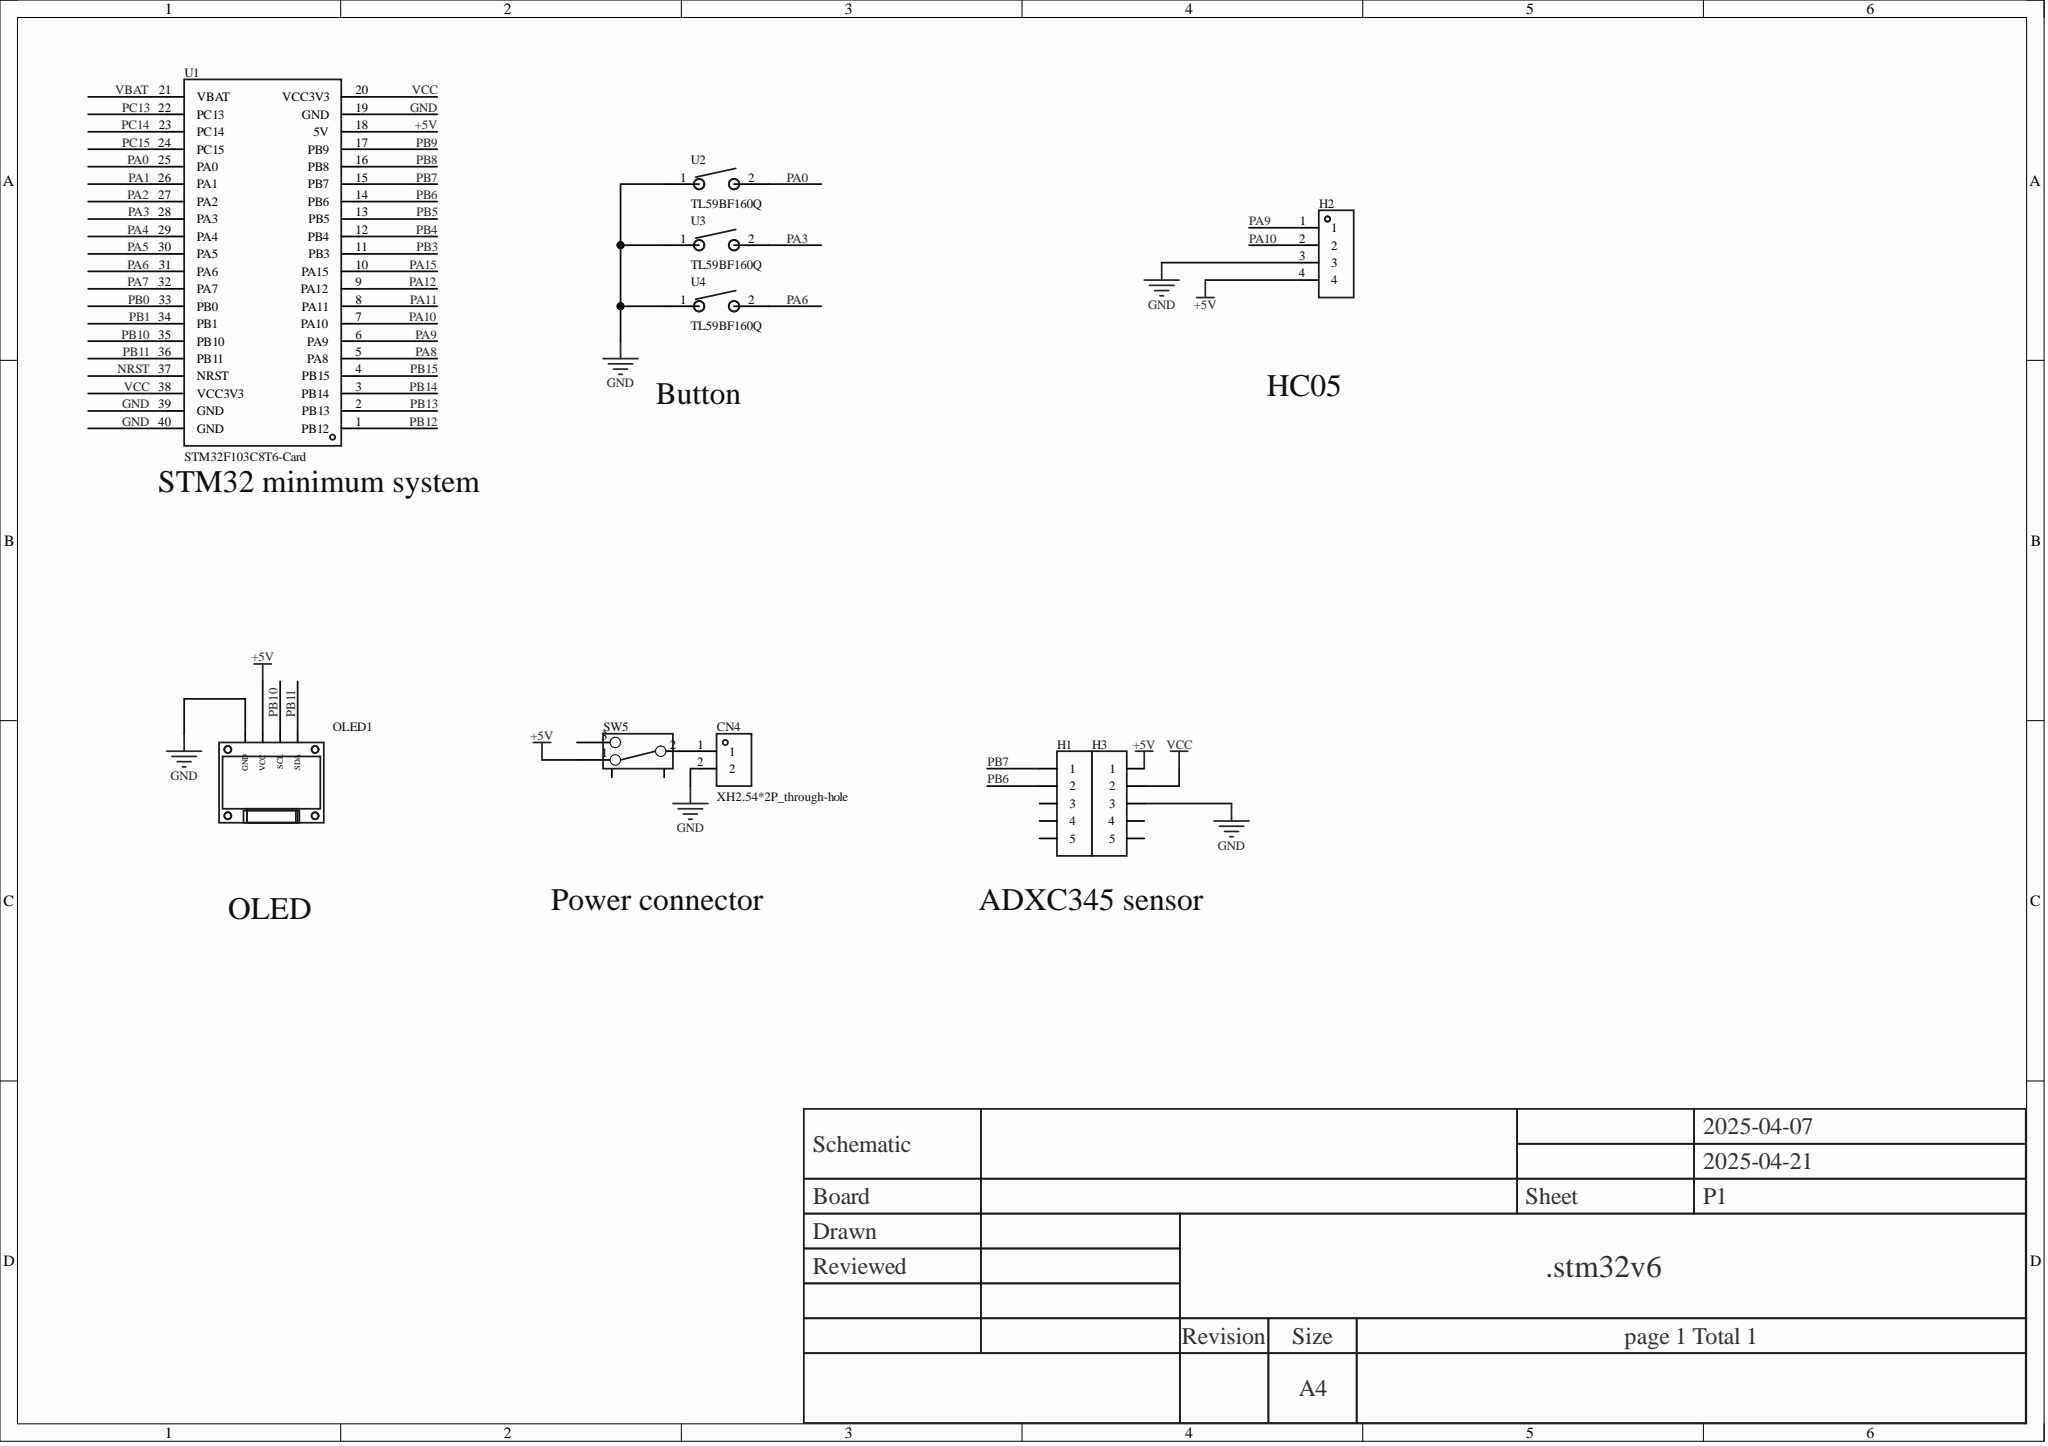Circuit board | Altium Designer | 10 parts | 13 nets
Bill of materials:
Comment,Description,Designator,Footprint,LibRef,Quantity
"XH2.54*2P_through-hole","","CN4","CONN-TH_2P-P2.50-XH2.54-2P","XH2.54*2P_直插","1"
"","","H1, H3","HDR-TH_5P-P2.54-V-F","HDR-F_2.54_1x5P","2"
"","","H2","HDR-TH_4P-P2.54-V-F","HDR-F_2.54_1x4P","1"
"","","OLED1","0.96OLED_4P","0.96OLED模块_4P","1"
"","","SW5","拨动开关","拨动开关_正","1"
"STM32F103C8T6-Card","","U1","CONN-TH_L53.3-W22.9_STM32F103C8T6-CARD","STM32F103C8T6-Card","1"
"TL59BF160Q","","U2, U3, U4","KEY-TH_L6.2-W6.2-P5.00","TL59BF160Q","3"
Netlist (Protel format):
[
CN4
CONN-TH_2P-P2.50-XH2.54-2P
XH2.54*2P_through-hole



]
[
H1
HDR-TH_5P-P2.54-V-F




]
[
H2
HDR-TH_4P-P2.54-V-F




]
[
H3
HDR-TH_5P-P2.54-V-F




]
[
OLED1
0.96OLED_4P




]
[
SW5
拨动开关




]
[
U1
CONN-TH_L53.3-W22.9_STM32F103C8T6-CARD
STM32F103C8T6-Card



]
[
U2
KEY-TH_L6.2-W6.2-P5.00
TL59BF160Q



]
[
U3
KEY-TH_L6.2-W6.2-P5.00
TL59BF160Q



]
[
U4
KEY-TH_L6.2-W6.2-P5.00
TL59BF160Q



]
(
VCC
H3-2
U1-20
U1-38
)
(
PB11
OLED1-4
U1-36
)
(
PB10
OLED1-3
U1-35
)
(
PB7
H1-1
U1-15
)
(
PB6
H1-2
U1-14
)
(
PA10
H2-2
U1-7
)
(
PA9
H2-1
U1-6
)
(
PA6
U1-31
U4-2
)
(
PA3
U1-28
U3-2
)
(
PA0
U1-25
U2-2
)
(
NetCN4_1
CN4-1
SW5-2
)
(
GND
CN4-2
H2-3
H3-3
OLED1-1
U1-19
U1-39
U1-40
U2-1
U3-1
U4-1
)
(
+5V
H2-4
H3-1
OLED1-2
SW5-1
U1-18
)